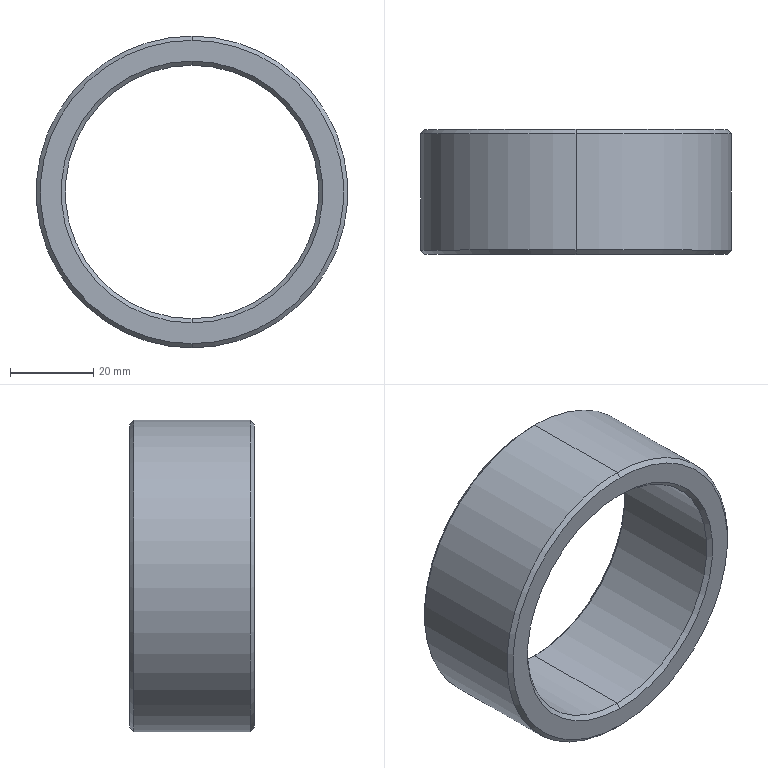Part | SolidWorks | features Chamfer 1, Extrusion 1 | 1 solid | 14 faces | box 75 x 30 x 75 mm | volume 44435 mm3 | cone 8 | cylinder 4 | plane 2 | commonest cylinder face diameters 61 x2 75 x2
STEP:
#1=CARTESIAN_POINT('',(0.,1.,30.5));
#2=VERTEX_POINT('',#1);
#3=CARTESIAN_POINT('',(0.,1.,-30.5));
#4=VERTEX_POINT('',#3);
#5=CARTESIAN_POINT('',(0.,1.,0.));
#6=DIRECTION('',(0.,-1.,0.));
#7=DIRECTION('',(0.,0.,1.));
#8=AXIS2_PLACEMENT_3D('',#5,#6,#7);
#9=CIRCLE('',#8,30.5);
#10=EDGE_CURVE('',#2,#4,#9,.T.);
#11=ORIENTED_EDGE('',*,*,#10,.F.);
#12=CARTESIAN_POINT('',(0.,0.,31.5));
#13=VERTEX_POINT('',#12);
#14=CARTESIAN_POINT('',(0.,0.,31.5));
#15=DIRECTION('',(0.,-0.7071,0.7071));
#16=VECTOR('',#15,1000.);
#17=LINE('',#14,#16);
#18=EDGE_CURVE('',#2,#13,#17,.T.);
#19=ORIENTED_EDGE('',*,*,#18,.T.);
#20=CARTESIAN_POINT('',(0.,0.,-31.5));
#21=VERTEX_POINT('',#20);
#22=CARTESIAN_POINT('',(0.,0.,0.));
#23=DIRECTION('',(0.,1.,0.));
#24=DIRECTION('',(0.,0.,1.));
#25=AXIS2_PLACEMENT_3D('',#22,#23,#24);
#26=CIRCLE('',#25,31.5);
#27=EDGE_CURVE('',#21,#13,#26,.T.);
#28=ORIENTED_EDGE('',*,*,#27,.F.);
#29=CARTESIAN_POINT('',(0.,0.,-31.5));
#30=DIRECTION('',(0.,-0.7071,-0.7071));
#31=VECTOR('',#30,1000.);
#32=LINE('',#29,#31);
#33=EDGE_CURVE('',#4,#21,#32,.T.);
#34=ORIENTED_EDGE('',*,*,#33,.F.);
#35=EDGE_LOOP('',(#11,#19,#28,#34));
#36=FACE_OUTER_BOUND('',#35,.T.);
#37=CARTESIAN_POINT('',(0.,0.,0.));
#38=DIRECTION('',(0.,-1.,0.));
#39=DIRECTION('',(0.,0.,-1.));
#40=AXIS2_PLACEMENT_3D('',#37,#38,#39);
#41=CONICAL_SURFACE('',#40,31.5,0.7854);
#42=ADVANCED_FACE('',(#36),#41,.F.);
#43=CARTESIAN_POINT('',(0.,29.,-30.5));
#44=VERTEX_POINT('',#43);
#45=CARTESIAN_POINT('',(0.,29.,30.5));
#46=VERTEX_POINT('',#45);
#47=CARTESIAN_POINT('',(0.,29.,0.));
#48=DIRECTION('',(0.,1.,0.));
#49=DIRECTION('',(0.,0.,1.));
#50=AXIS2_PLACEMENT_3D('',#47,#48,#49);
#51=CIRCLE('',#50,30.5);
#52=EDGE_CURVE('',#44,#46,#51,.T.);
#53=ORIENTED_EDGE('',*,*,#52,.F.);
#54=CARTESIAN_POINT('',(0.,30.,-31.5));
#55=VERTEX_POINT('',#54);
#56=CARTESIAN_POINT('',(0.,29.,-30.5));
#57=DIRECTION('',(0.,0.7071,-0.7071));
#58=VECTOR('',#57,1000.);
#59=LINE('',#56,#58);
#60=EDGE_CURVE('',#44,#55,#59,.T.);
#61=ORIENTED_EDGE('',*,*,#60,.T.);
#62=CARTESIAN_POINT('',(0.,30.,31.5));
#63=VERTEX_POINT('',#62);
#64=CARTESIAN_POINT('',(0.,30.,0.));
#65=DIRECTION('',(0.,-1.,0.));
#66=DIRECTION('',(0.,0.,1.));
#67=AXIS2_PLACEMENT_3D('',#64,#65,#66);
#68=CIRCLE('',#67,31.5);
#69=EDGE_CURVE('',#63,#55,#68,.T.);
#70=ORIENTED_EDGE('',*,*,#69,.F.);
#71=CARTESIAN_POINT('',(0.,29.,30.5));
#72=DIRECTION('',(0.,0.7071,0.7071));
#73=VECTOR('',#72,1000.);
#74=LINE('',#71,#73);
#75=EDGE_CURVE('',#46,#63,#74,.T.);
#76=ORIENTED_EDGE('',*,*,#75,.F.);
#77=EDGE_LOOP('',(#53,#61,#70,#76));
#78=FACE_OUTER_BOUND('',#77,.T.);
#79=CARTESIAN_POINT('',(0.,29.,0.));
#80=DIRECTION('',(0.,1.,0.));
#81=DIRECTION('',(0.,0.,1.));
#82=AXIS2_PLACEMENT_3D('',#79,#80,#81);
#83=CONICAL_SURFACE('',#82,30.5,0.7854);
#84=ADVANCED_FACE('',(#78),#83,.F.);
#85=CARTESIAN_POINT('',(0.,0.,-36.5));
#86=VERTEX_POINT('',#85);
#87=CARTESIAN_POINT('',(0.,0.,36.5));
#88=VERTEX_POINT('',#87);
#89=CARTESIAN_POINT('',(0.,0.,0.));
#90=DIRECTION('',(0.,-1.,0.));
#91=DIRECTION('',(0.,0.,1.));
#92=AXIS2_PLACEMENT_3D('',#89,#90,#91);
#93=CIRCLE('',#92,36.5);
#94=EDGE_CURVE('',#86,#88,#93,.T.);
#95=ORIENTED_EDGE('',*,*,#94,.F.);
#96=CARTESIAN_POINT('',(0.,1.,-37.5));
#97=VERTEX_POINT('',#96);
#98=CARTESIAN_POINT('',(0.,1.,-37.5));
#99=DIRECTION('',(0.,0.7071,-0.7071));
#100=VECTOR('',#99,1000.);
#101=LINE('',#98,#100);
#102=EDGE_CURVE('',#86,#97,#101,.T.);
#103=ORIENTED_EDGE('',*,*,#102,.T.);
#104=CARTESIAN_POINT('',(0.,1.,37.5));
#105=VERTEX_POINT('',#104);
#106=CARTESIAN_POINT('',(0.,1.,0.));
#107=DIRECTION('',(0.,1.,0.));
#108=DIRECTION('',(0.,0.,1.));
#109=AXIS2_PLACEMENT_3D('',#106,#107,#108);
#110=CIRCLE('',#109,37.5);
#111=EDGE_CURVE('',#105,#97,#110,.T.);
#112=ORIENTED_EDGE('',*,*,#111,.F.);
#113=CARTESIAN_POINT('',(0.,1.,37.5));
#114=DIRECTION('',(0.,0.7071,0.7071));
#115=VECTOR('',#114,1000.);
#116=LINE('',#113,#115);
#117=EDGE_CURVE('',#88,#105,#116,.T.);
#118=ORIENTED_EDGE('',*,*,#117,.F.);
#119=EDGE_LOOP('',(#95,#103,#112,#118));
#120=FACE_OUTER_BOUND('',#119,.T.);
#121=CARTESIAN_POINT('',(0.,1.,0.));
#122=DIRECTION('',(0.,1.,0.));
#123=DIRECTION('',(0.,0.,1.));
#124=AXIS2_PLACEMENT_3D('',#121,#122,#123);
#125=CONICAL_SURFACE('',#124,37.5,0.7854);
#126=ADVANCED_FACE('',(#120),#125,.T.);
#127=CARTESIAN_POINT('',(0.,30.,36.5));
#128=VERTEX_POINT('',#127);
#129=CARTESIAN_POINT('',(0.,30.,-36.5));
#130=VERTEX_POINT('',#129);
#131=CARTESIAN_POINT('',(0.,30.,0.));
#132=DIRECTION('',(0.,1.,0.));
#133=DIRECTION('',(0.,0.,1.));
#134=AXIS2_PLACEMENT_3D('',#131,#132,#133);
#135=CIRCLE('',#134,36.5);
#136=EDGE_CURVE('',#128,#130,#135,.T.);
#137=ORIENTED_EDGE('',*,*,#136,.F.);
#138=CARTESIAN_POINT('',(0.,29.,37.5));
#139=VERTEX_POINT('',#138);
#140=CARTESIAN_POINT('',(0.,30.,36.5));
#141=DIRECTION('',(0.,-0.7071,0.7071));
#142=VECTOR('',#141,1000.);
#143=LINE('',#140,#142);
#144=EDGE_CURVE('',#128,#139,#143,.T.);
#145=ORIENTED_EDGE('',*,*,#144,.T.);
#146=CARTESIAN_POINT('',(0.,29.,-37.5));
#147=VERTEX_POINT('',#146);
#148=CARTESIAN_POINT('',(0.,29.,0.));
#149=DIRECTION('',(0.,-1.,0.));
#150=DIRECTION('',(0.,0.,1.));
#151=AXIS2_PLACEMENT_3D('',#148,#149,#150);
#152=CIRCLE('',#151,37.5);
#153=EDGE_CURVE('',#147,#139,#152,.T.);
#154=ORIENTED_EDGE('',*,*,#153,.F.);
#155=CARTESIAN_POINT('',(0.,30.,-36.5));
#156=DIRECTION('',(0.,-0.7071,-0.7071));
#157=VECTOR('',#156,1000.);
#158=LINE('',#155,#157);
#159=EDGE_CURVE('',#130,#147,#158,.T.);
#160=ORIENTED_EDGE('',*,*,#159,.F.);
#161=EDGE_LOOP('',(#137,#145,#154,#160));
#162=FACE_OUTER_BOUND('',#161,.T.);
#163=CARTESIAN_POINT('',(0.,30.,0.));
#164=DIRECTION('',(0.,-1.,0.));
#165=DIRECTION('',(0.,0.,-1.));
#166=AXIS2_PLACEMENT_3D('',#163,#164,#165);
#167=CONICAL_SURFACE('',#166,36.5,0.7854);
#168=ADVANCED_FACE('',(#162),#167,.T.);
#169=ORIENTED_EDGE('',*,*,#52,.T.);
#170=CARTESIAN_POINT('',(0.,30.,30.5));
#171=DIRECTION('',(0.,-1.,0.));
#172=VECTOR('',#171,1000.);
#173=LINE('',#170,#172);
#174=EDGE_CURVE('',#46,#2,#173,.T.);
#175=ORIENTED_EDGE('',*,*,#174,.T.);
#176=ORIENTED_EDGE('',*,*,#10,.T.);
#177=CARTESIAN_POINT('',(0.,30.,-30.5));
#178=DIRECTION('',(0.,-1.,0.));
#179=VECTOR('',#178,1000.);
#180=LINE('',#177,#179);
#181=EDGE_CURVE('',#44,#4,#180,.T.);
#182=ORIENTED_EDGE('',*,*,#181,.F.);
#183=EDGE_LOOP('',(#169,#175,#176,#182));
#184=FACE_OUTER_BOUND('',#183,.T.);
#185=CARTESIAN_POINT('',(0.,30.,0.));
#186=DIRECTION('',(0.,-1.,0.));
#187=DIRECTION('',(0.,0.,-1.));
#188=AXIS2_PLACEMENT_3D('',#185,#186,#187);
#189=CYLINDRICAL_SURFACE('',#188,30.5);
#190=ADVANCED_FACE('',(#184),#189,.F.);
#191=ORIENTED_EDGE('',*,*,#153,.T.);
#192=CARTESIAN_POINT('',(0.,30.,37.5));
#193=DIRECTION('',(0.,-1.,0.));
#194=VECTOR('',#193,1000.);
#195=LINE('',#192,#194);
#196=EDGE_CURVE('',#139,#105,#195,.T.);
#197=ORIENTED_EDGE('',*,*,#196,.T.);
#198=ORIENTED_EDGE('',*,*,#111,.T.);
#199=CARTESIAN_POINT('',(0.,30.,-37.5));
#200=DIRECTION('',(0.,-1.,0.));
#201=VECTOR('',#200,1000.);
#202=LINE('',#199,#201);
#203=EDGE_CURVE('',#147,#97,#202,.T.);
#204=ORIENTED_EDGE('',*,*,#203,.F.);
#205=EDGE_LOOP('',(#191,#197,#198,#204));
#206=FACE_OUTER_BOUND('',#205,.T.);
#207=CARTESIAN_POINT('',(0.,30.,0.));
#208=DIRECTION('',(0.,-1.,0.));
#209=DIRECTION('',(0.,0.,-1.));
#210=AXIS2_PLACEMENT_3D('',#207,#208,#209);
#211=CYLINDRICAL_SURFACE('',#210,37.5);
#212=ADVANCED_FACE('',(#206),#211,.T.);
#213=CARTESIAN_POINT('',(0.,30.,0.));
#214=DIRECTION('',(0.,1.,0.));
#215=DIRECTION('',(0.,0.,1.));
#216=AXIS2_PLACEMENT_3D('',#213,#214,#215);
#217=CIRCLE('',#216,36.5);
#218=EDGE_CURVE('',#130,#128,#217,.T.);
#219=ORIENTED_EDGE('',*,*,#218,.T.);
#220=ORIENTED_EDGE('',*,*,#136,.T.);
#221=EDGE_LOOP('',(#219,#220));
#222=FACE_OUTER_BOUND('',#221,.T.);
#223=ORIENTED_EDGE('',*,*,#69,.T.);
#224=CARTESIAN_POINT('',(0.,30.,0.));
#225=DIRECTION('',(0.,-1.,0.));
#226=DIRECTION('',(0.,0.,1.));
#227=AXIS2_PLACEMENT_3D('',#224,#225,#226);
#228=CIRCLE('',#227,31.5);
#229=EDGE_CURVE('',#55,#63,#228,.T.);
#230=ORIENTED_EDGE('',*,*,#229,.T.);
#231=EDGE_LOOP('',(#223,#230));
#232=FACE_BOUND('',#231,.T.);
#233=CARTESIAN_POINT('',(0.,30.,0.));
#234=DIRECTION('',(0.,1.,0.));
#235=DIRECTION('',(0.,0.,1.));
#236=AXIS2_PLACEMENT_3D('',#233,#234,#235);
#237=PLANE('',#236);
#238=ADVANCED_FACE('',(#222,#232),#237,.T.);
#239=CARTESIAN_POINT('',(0.,0.,0.));
#240=DIRECTION('',(0.,-1.,0.));
#241=DIRECTION('',(0.,0.,1.));
#242=AXIS2_PLACEMENT_3D('',#239,#240,#241);
#243=CIRCLE('',#242,36.5);
#244=EDGE_CURVE('',#88,#86,#243,.T.);
#245=ORIENTED_EDGE('',*,*,#244,.T.);
#246=ORIENTED_EDGE('',*,*,#94,.T.);
#247=EDGE_LOOP('',(#245,#246));
#248=FACE_OUTER_BOUND('',#247,.T.);
#249=ORIENTED_EDGE('',*,*,#27,.T.);
#250=CARTESIAN_POINT('',(0.,0.,0.));
#251=DIRECTION('',(0.,1.,0.));
#252=DIRECTION('',(0.,0.,1.));
#253=AXIS2_PLACEMENT_3D('',#250,#251,#252);
#254=CIRCLE('',#253,31.5);
#255=EDGE_CURVE('',#13,#21,#254,.T.);
#256=ORIENTED_EDGE('',*,*,#255,.T.);
#257=EDGE_LOOP('',(#249,#256));
#258=FACE_BOUND('',#257,.T.);
#259=CARTESIAN_POINT('',(0.,0.,0.));
#260=DIRECTION('',(0.,1.,0.));
#261=DIRECTION('',(0.,0.,1.));
#262=AXIS2_PLACEMENT_3D('',#259,#260,#261);
#263=PLANE('',#262);
#264=ADVANCED_FACE('',(#248,#258),#263,.F.);
#265=ORIENTED_EDGE('',*,*,#196,.F.);
#266=CARTESIAN_POINT('',(0.,29.,0.));
#267=DIRECTION('',(0.,-1.,0.));
#268=DIRECTION('',(0.,0.,1.));
#269=AXIS2_PLACEMENT_3D('',#266,#267,#268);
#270=CIRCLE('',#269,37.5);
#271=EDGE_CURVE('',#139,#147,#270,.T.);
#272=ORIENTED_EDGE('',*,*,#271,.T.);
#273=ORIENTED_EDGE('',*,*,#203,.T.);
#274=CARTESIAN_POINT('',(0.,1.,0.));
#275=DIRECTION('',(0.,1.,0.));
#276=DIRECTION('',(0.,0.,1.));
#277=AXIS2_PLACEMENT_3D('',#274,#275,#276);
#278=CIRCLE('',#277,37.5);
#279=EDGE_CURVE('',#97,#105,#278,.T.);
#280=ORIENTED_EDGE('',*,*,#279,.T.);
#281=EDGE_LOOP('',(#265,#272,#273,#280));
#282=FACE_OUTER_BOUND('',#281,.T.);
#283=CARTESIAN_POINT('',(0.,30.,0.));
#284=DIRECTION('',(0.,-1.,0.));
#285=DIRECTION('',(0.,0.,-1.));
#286=AXIS2_PLACEMENT_3D('',#283,#284,#285);
#287=CYLINDRICAL_SURFACE('',#286,37.5);
#288=ADVANCED_FACE('',(#282),#287,.T.);
#289=ORIENTED_EDGE('',*,*,#174,.F.);
#290=CARTESIAN_POINT('',(0.,29.,0.));
#291=DIRECTION('',(0.,1.,0.));
#292=DIRECTION('',(0.,0.,1.));
#293=AXIS2_PLACEMENT_3D('',#290,#291,#292);
#294=CIRCLE('',#293,30.5);
#295=EDGE_CURVE('',#46,#44,#294,.T.);
#296=ORIENTED_EDGE('',*,*,#295,.T.);
#297=ORIENTED_EDGE('',*,*,#181,.T.);
#298=CARTESIAN_POINT('',(0.,1.,0.));
#299=DIRECTION('',(0.,-1.,0.));
#300=DIRECTION('',(0.,0.,1.));
#301=AXIS2_PLACEMENT_3D('',#298,#299,#300);
#302=CIRCLE('',#301,30.5);
#303=EDGE_CURVE('',#4,#2,#302,.T.);
#304=ORIENTED_EDGE('',*,*,#303,.T.);
#305=EDGE_LOOP('',(#289,#296,#297,#304));
#306=FACE_OUTER_BOUND('',#305,.T.);
#307=CARTESIAN_POINT('',(0.,30.,0.));
#308=DIRECTION('',(0.,-1.,0.));
#309=DIRECTION('',(0.,0.,-1.));
#310=AXIS2_PLACEMENT_3D('',#307,#308,#309);
#311=CYLINDRICAL_SURFACE('',#310,30.5);
#312=ADVANCED_FACE('',(#306),#311,.F.);
#313=ORIENTED_EDGE('',*,*,#144,.F.);
#314=ORIENTED_EDGE('',*,*,#218,.F.);
#315=ORIENTED_EDGE('',*,*,#159,.T.);
#316=ORIENTED_EDGE('',*,*,#271,.F.);
#317=EDGE_LOOP('',(#313,#314,#315,#316));
#318=FACE_OUTER_BOUND('',#317,.T.);
#319=CARTESIAN_POINT('',(0.,30.,0.));
#320=DIRECTION('',(0.,-1.,0.));
#321=DIRECTION('',(0.,0.,-1.));
#322=AXIS2_PLACEMENT_3D('',#319,#320,#321);
#323=CONICAL_SURFACE('',#322,36.5,0.7854);
#324=ADVANCED_FACE('',(#318),#323,.T.);
#325=ORIENTED_EDGE('',*,*,#102,.F.);
#326=ORIENTED_EDGE('',*,*,#244,.F.);
#327=ORIENTED_EDGE('',*,*,#117,.T.);
#328=ORIENTED_EDGE('',*,*,#279,.F.);
#329=EDGE_LOOP('',(#325,#326,#327,#328));
#330=FACE_OUTER_BOUND('',#329,.T.);
#331=CARTESIAN_POINT('',(0.,1.,0.));
#332=DIRECTION('',(0.,1.,0.));
#333=DIRECTION('',(0.,0.,1.));
#334=AXIS2_PLACEMENT_3D('',#331,#332,#333);
#335=CONICAL_SURFACE('',#334,37.5,0.7854);
#336=ADVANCED_FACE('',(#330),#335,.T.);
#337=ORIENTED_EDGE('',*,*,#60,.F.);
#338=ORIENTED_EDGE('',*,*,#295,.F.);
#339=ORIENTED_EDGE('',*,*,#75,.T.);
#340=ORIENTED_EDGE('',*,*,#229,.F.);
#341=EDGE_LOOP('',(#337,#338,#339,#340));
#342=FACE_OUTER_BOUND('',#341,.T.);
#343=CARTESIAN_POINT('',(0.,29.,0.));
#344=DIRECTION('',(0.,1.,0.));
#345=DIRECTION('',(0.,0.,1.));
#346=AXIS2_PLACEMENT_3D('',#343,#344,#345);
#347=CONICAL_SURFACE('',#346,30.5,0.7854);
#348=ADVANCED_FACE('',(#342),#347,.F.);
#349=ORIENTED_EDGE('',*,*,#18,.F.);
#350=ORIENTED_EDGE('',*,*,#303,.F.);
#351=ORIENTED_EDGE('',*,*,#33,.T.);
#352=ORIENTED_EDGE('',*,*,#255,.F.);
#353=EDGE_LOOP('',(#349,#350,#351,#352));
#354=FACE_OUTER_BOUND('',#353,.T.);
#355=CARTESIAN_POINT('',(0.,0.,0.));
#356=DIRECTION('',(0.,-1.,0.));
#357=DIRECTION('',(0.,0.,-1.));
#358=AXIS2_PLACEMENT_3D('',#355,#356,#357);
#359=CONICAL_SURFACE('',#358,31.5,0.7854);
#360=ADVANCED_FACE('',(#354),#359,.F.);
#361=CLOSED_SHELL('',(#42,#84,#126,#168,#190,#212,#238,#264,#288,#312,#324,#336,#348,#360));
#362=MANIFOLD_SOLID_BREP('',#361);
#363=CARTESIAN_POINT('',(0.,0.,0.));
#364=DIRECTION('',(0.,0.,1.));
#365=DIRECTION('',(1.,0.,0.));
#366=AXIS2_PLACEMENT_3D('',#363,#364,#365);
#367=(LENGTH_UNIT()NAMED_UNIT(*)SI_UNIT(.MILLI.,.METRE.));
#368=UNCERTAINTY_MEASURE_WITH_UNIT(LENGTH_MEASURE(0.00001),#367,'','');
#369=(NAMED_UNIT(*)PLANE_ANGLE_UNIT()SI_UNIT($,.RADIAN.));
#370=(NAMED_UNIT(*)SI_UNIT($,.STERADIAN.)SOLID_ANGLE_UNIT());
#371=(GEOMETRIC_REPRESENTATION_CONTEXT(3)GLOBAL_UNCERTAINTY_ASSIGNED_CONTEXT((#368))GLOBAL_UNIT_ASSIGNED_CONTEXT((#367,#369,#370))REPRESENTATION_CONTEXT('',''));
#372=ADVANCED_BREP_SHAPE_REPRESENTATION('',(#362,#366),#371);